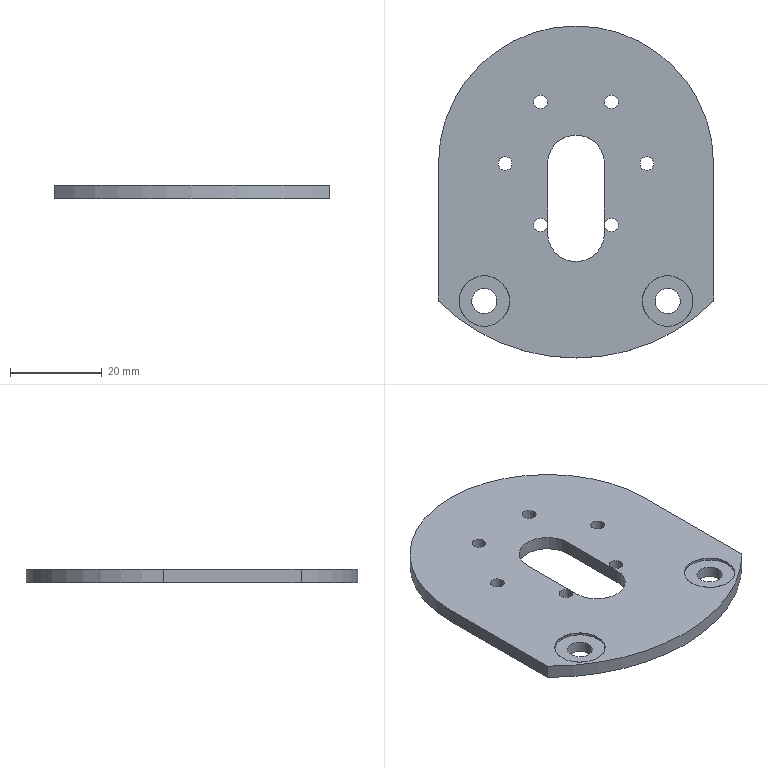Part | SolidWorks | features Extrusion 1, HoleWzd 1, ICE 1 | 1 solid | 36 faces | box 60 x 72.426 x 3 mm | volume 9913 mm3 | cylinder 24 | plane 8 | cone 4 | commonest cylinder face diameters 3 x12 5.5 x4 11 x4 12.4 x2 60 x1 84.853 x1
STEP:
#1=CARTESIAN_POINT('',(-25.5,-30.,2.975));
#2=VERTEX_POINT('',#1);
#3=CARTESIAN_POINT('',(-14.5,-30.,2.975));
#4=VERTEX_POINT('',#3);
#5=CARTESIAN_POINT('',(-20.,-30.,2.975));
#6=DIRECTION('',(0.,0.,1.));
#7=DIRECTION('',(1.,0.,0.));
#8=AXIS2_PLACEMENT_3D('',#5,#6,#7);
#9=CIRCLE('',#8,5.5);
#10=EDGE_CURVE('',#2,#4,#9,.T.);
#11=ORIENTED_EDGE('',*,*,#10,.F.);
#12=CARTESIAN_POINT('',(-25.525,-30.,3.));
#13=VERTEX_POINT('',#12);
#14=CARTESIAN_POINT('',(-25.525,-30.,3.));
#15=DIRECTION('',(-0.7071,0.,0.7071));
#16=VECTOR('',#15,1000.);
#17=LINE('',#14,#16);
#18=EDGE_CURVE('',#2,#13,#17,.T.);
#19=ORIENTED_EDGE('',*,*,#18,.T.);
#20=CARTESIAN_POINT('',(-14.475,-30.,3.));
#21=VERTEX_POINT('',#20);
#22=CARTESIAN_POINT('',(-20.,-30.,3.));
#23=DIRECTION('',(0.,0.,1.));
#24=DIRECTION('',(1.,0.,0.));
#25=AXIS2_PLACEMENT_3D('',#22,#23,#24);
#26=CIRCLE('',#25,5.525);
#27=EDGE_CURVE('',#13,#21,#26,.T.);
#28=ORIENTED_EDGE('',*,*,#27,.T.);
#29=CARTESIAN_POINT('',(-14.475,-30.,3.));
#30=DIRECTION('',(0.7071,0.,0.7071));
#31=VECTOR('',#30,1000.);
#32=LINE('',#29,#31);
#33=EDGE_CURVE('',#4,#21,#32,.T.);
#34=ORIENTED_EDGE('',*,*,#33,.F.);
#35=EDGE_LOOP('',(#11,#19,#28,#34));
#36=FACE_OUTER_BOUND('',#35,.T.);
#37=CARTESIAN_POINT('',(-20.,-30.,3.));
#38=DIRECTION('',(0.,0.,1.));
#39=DIRECTION('',(1.,0.,0.));
#40=AXIS2_PLACEMENT_3D('',#37,#38,#39);
#41=CONICAL_SURFACE('',#40,5.525,0.7854);
#42=ADVANCED_FACE('',(#36),#41,.F.);
#43=CARTESIAN_POINT('',(-25.5,-30.,2.5));
#44=VERTEX_POINT('',#43);
#45=CARTESIAN_POINT('',(-14.5,-30.,2.5));
#46=VERTEX_POINT('',#45);
#47=CARTESIAN_POINT('',(-20.,-30.,2.5));
#48=DIRECTION('',(0.,0.,1.));
#49=DIRECTION('',(1.,0.,0.));
#50=AXIS2_PLACEMENT_3D('',#47,#48,#49);
#51=CIRCLE('',#50,5.5);
#52=EDGE_CURVE('',#44,#46,#51,.T.);
#53=ORIENTED_EDGE('',*,*,#52,.F.);
#54=CARTESIAN_POINT('',(-25.5,-30.,3.));
#55=DIRECTION('',(0.,0.,1.));
#56=VECTOR('',#55,1000.);
#57=LINE('',#54,#56);
#58=EDGE_CURVE('',#44,#2,#57,.T.);
#59=ORIENTED_EDGE('',*,*,#58,.T.);
#60=ORIENTED_EDGE('',*,*,#10,.T.);
#61=CARTESIAN_POINT('',(-14.5,-30.,3.));
#62=DIRECTION('',(0.,0.,1.));
#63=VECTOR('',#62,1000.);
#64=LINE('',#61,#63);
#65=EDGE_CURVE('',#46,#4,#64,.T.);
#66=ORIENTED_EDGE('',*,*,#65,.F.);
#67=EDGE_LOOP('',(#53,#59,#60,#66));
#68=FACE_OUTER_BOUND('',#67,.T.);
#69=CARTESIAN_POINT('',(-20.,-30.,3.));
#70=DIRECTION('',(0.,0.,1.));
#71=DIRECTION('',(1.,0.,0.));
#72=AXIS2_PLACEMENT_3D('',#69,#70,#71);
#73=CYLINDRICAL_SURFACE('',#72,5.5);
#74=ADVANCED_FACE('',(#68),#73,.F.);
#75=CARTESIAN_POINT('',(-22.75,-30.,0.));
#76=VERTEX_POINT('',#75);
#77=CARTESIAN_POINT('',(-17.25,-30.,0.));
#78=VERTEX_POINT('',#77);
#79=CARTESIAN_POINT('',(-20.,-30.,0.));
#80=DIRECTION('',(0.,0.,1.));
#81=DIRECTION('',(1.,0.,0.));
#82=AXIS2_PLACEMENT_3D('',#79,#80,#81);
#83=CIRCLE('',#82,2.75);
#84=EDGE_CURVE('',#76,#78,#83,.T.);
#85=ORIENTED_EDGE('',*,*,#84,.F.);
#86=CARTESIAN_POINT('',(-22.75,-30.,2.5));
#87=VERTEX_POINT('',#86);
#88=CARTESIAN_POINT('',(-22.75,-30.,3.));
#89=DIRECTION('',(0.,0.,1.));
#90=VECTOR('',#89,1000.);
#91=LINE('',#88,#90);
#92=EDGE_CURVE('',#76,#87,#91,.T.);
#93=ORIENTED_EDGE('',*,*,#92,.T.);
#94=CARTESIAN_POINT('',(-17.25,-30.,2.5));
#95=VERTEX_POINT('',#94);
#96=CARTESIAN_POINT('',(-20.,-30.,2.5));
#97=DIRECTION('',(0.,0.,1.));
#98=DIRECTION('',(1.,0.,0.));
#99=AXIS2_PLACEMENT_3D('',#96,#97,#98);
#100=CIRCLE('',#99,2.75);
#101=EDGE_CURVE('',#87,#95,#100,.T.);
#102=ORIENTED_EDGE('',*,*,#101,.T.);
#103=CARTESIAN_POINT('',(-17.25,-30.,3.));
#104=DIRECTION('',(0.,0.,1.));
#105=VECTOR('',#104,1000.);
#106=LINE('',#103,#105);
#107=EDGE_CURVE('',#78,#95,#106,.T.);
#108=ORIENTED_EDGE('',*,*,#107,.F.);
#109=EDGE_LOOP('',(#85,#93,#102,#108));
#110=FACE_OUTER_BOUND('',#109,.T.);
#111=CARTESIAN_POINT('',(-20.,-30.,3.));
#112=DIRECTION('',(0.,0.,1.));
#113=DIRECTION('',(1.,0.,0.));
#114=AXIS2_PLACEMENT_3D('',#111,#112,#113);
#115=CYLINDRICAL_SURFACE('',#114,2.75);
#116=ADVANCED_FACE('',(#110),#115,.F.);
#117=CARTESIAN_POINT('',(14.5,-30.,2.975));
#118=VERTEX_POINT('',#117);
#119=CARTESIAN_POINT('',(25.5,-30.,2.975));
#120=VERTEX_POINT('',#119);
#121=CARTESIAN_POINT('',(20.,-30.,2.975));
#122=DIRECTION('',(0.,0.,1.));
#123=DIRECTION('',(1.,0.,0.));
#124=AXIS2_PLACEMENT_3D('',#121,#122,#123);
#125=CIRCLE('',#124,5.5);
#126=EDGE_CURVE('',#118,#120,#125,.T.);
#127=ORIENTED_EDGE('',*,*,#126,.F.);
#128=CARTESIAN_POINT('',(14.475,-30.,3.));
#129=VERTEX_POINT('',#128);
#130=CARTESIAN_POINT('',(14.475,-30.,3.));
#131=DIRECTION('',(-0.7071,0.,0.7071));
#132=VECTOR('',#131,1000.);
#133=LINE('',#130,#132);
#134=EDGE_CURVE('',#118,#129,#133,.T.);
#135=ORIENTED_EDGE('',*,*,#134,.T.);
#136=CARTESIAN_POINT('',(25.525,-30.,3.));
#137=VERTEX_POINT('',#136);
#138=CARTESIAN_POINT('',(20.,-30.,3.));
#139=DIRECTION('',(0.,0.,1.));
#140=DIRECTION('',(1.,0.,0.));
#141=AXIS2_PLACEMENT_3D('',#138,#139,#140);
#142=CIRCLE('',#141,5.525);
#143=EDGE_CURVE('',#129,#137,#142,.T.);
#144=ORIENTED_EDGE('',*,*,#143,.T.);
#145=CARTESIAN_POINT('',(25.525,-30.,3.));
#146=DIRECTION('',(0.7071,0.,0.7071));
#147=VECTOR('',#146,1000.);
#148=LINE('',#145,#147);
#149=EDGE_CURVE('',#120,#137,#148,.T.);
#150=ORIENTED_EDGE('',*,*,#149,.F.);
#151=EDGE_LOOP('',(#127,#135,#144,#150));
#152=FACE_OUTER_BOUND('',#151,.T.);
#153=CARTESIAN_POINT('',(20.,-30.,3.));
#154=DIRECTION('',(0.,0.,1.));
#155=DIRECTION('',(1.,0.,0.));
#156=AXIS2_PLACEMENT_3D('',#153,#154,#155);
#157=CONICAL_SURFACE('',#156,5.525,0.7854);
#158=ADVANCED_FACE('',(#152),#157,.F.);
#159=CARTESIAN_POINT('',(14.5,-30.,2.5));
#160=VERTEX_POINT('',#159);
#161=CARTESIAN_POINT('',(25.5,-30.,2.5));
#162=VERTEX_POINT('',#161);
#163=CARTESIAN_POINT('',(20.,-30.,2.5));
#164=DIRECTION('',(0.,0.,1.));
#165=DIRECTION('',(1.,0.,0.));
#166=AXIS2_PLACEMENT_3D('',#163,#164,#165);
#167=CIRCLE('',#166,5.5);
#168=EDGE_CURVE('',#160,#162,#167,.T.);
#169=ORIENTED_EDGE('',*,*,#168,.F.);
#170=CARTESIAN_POINT('',(14.5,-30.,3.));
#171=DIRECTION('',(0.,0.,1.));
#172=VECTOR('',#171,1000.);
#173=LINE('',#170,#172);
#174=EDGE_CURVE('',#160,#118,#173,.T.);
#175=ORIENTED_EDGE('',*,*,#174,.T.);
#176=ORIENTED_EDGE('',*,*,#126,.T.);
#177=CARTESIAN_POINT('',(25.5,-30.,3.));
#178=DIRECTION('',(0.,0.,1.));
#179=VECTOR('',#178,1000.);
#180=LINE('',#177,#179);
#181=EDGE_CURVE('',#162,#120,#180,.T.);
#182=ORIENTED_EDGE('',*,*,#181,.F.);
#183=EDGE_LOOP('',(#169,#175,#176,#182));
#184=FACE_OUTER_BOUND('',#183,.T.);
#185=CARTESIAN_POINT('',(20.,-30.,3.));
#186=DIRECTION('',(0.,0.,1.));
#187=DIRECTION('',(1.,0.,0.));
#188=AXIS2_PLACEMENT_3D('',#185,#186,#187);
#189=CYLINDRICAL_SURFACE('',#188,5.5);
#190=ADVANCED_FACE('',(#184),#189,.F.);
#191=CARTESIAN_POINT('',(17.25,-30.,0.));
#192=VERTEX_POINT('',#191);
#193=CARTESIAN_POINT('',(22.75,-30.,0.));
#194=VERTEX_POINT('',#193);
#195=CARTESIAN_POINT('',(20.,-30.,0.));
#196=DIRECTION('',(0.,0.,1.));
#197=DIRECTION('',(1.,0.,0.));
#198=AXIS2_PLACEMENT_3D('',#195,#196,#197);
#199=CIRCLE('',#198,2.75);
#200=EDGE_CURVE('',#192,#194,#199,.T.);
#201=ORIENTED_EDGE('',*,*,#200,.F.);
#202=CARTESIAN_POINT('',(17.25,-30.,2.5));
#203=VERTEX_POINT('',#202);
#204=CARTESIAN_POINT('',(17.25,-30.,3.));
#205=DIRECTION('',(0.,0.,1.));
#206=VECTOR('',#205,1000.);
#207=LINE('',#204,#206);
#208=EDGE_CURVE('',#192,#203,#207,.T.);
#209=ORIENTED_EDGE('',*,*,#208,.T.);
#210=CARTESIAN_POINT('',(22.75,-30.,2.5));
#211=VERTEX_POINT('',#210);
#212=CARTESIAN_POINT('',(20.,-30.,2.5));
#213=DIRECTION('',(0.,0.,1.));
#214=DIRECTION('',(1.,0.,0.));
#215=AXIS2_PLACEMENT_3D('',#212,#213,#214);
#216=CIRCLE('',#215,2.75);
#217=EDGE_CURVE('',#203,#211,#216,.T.);
#218=ORIENTED_EDGE('',*,*,#217,.T.);
#219=CARTESIAN_POINT('',(22.75,-30.,3.));
#220=DIRECTION('',(0.,0.,1.));
#221=VECTOR('',#220,1000.);
#222=LINE('',#219,#221);
#223=EDGE_CURVE('',#194,#211,#222,.T.);
#224=ORIENTED_EDGE('',*,*,#223,.F.);
#225=EDGE_LOOP('',(#201,#209,#218,#224));
#226=FACE_OUTER_BOUND('',#225,.T.);
#227=CARTESIAN_POINT('',(20.,-30.,3.));
#228=DIRECTION('',(0.,0.,1.));
#229=DIRECTION('',(1.,0.,0.));
#230=AXIS2_PLACEMENT_3D('',#227,#228,#229);
#231=CYLINDRICAL_SURFACE('',#230,2.75);
#232=ADVANCED_FACE('',(#226),#231,.F.);
#233=CARTESIAN_POINT('',(-16.964,0.,0.));
#234=VERTEX_POINT('',#233);
#235=CARTESIAN_POINT('',(-13.964,0.,0.));
#236=VERTEX_POINT('',#235);
#237=CARTESIAN_POINT('',(-15.464,0.,0.));
#238=DIRECTION('',(0.,0.,1.));
#239=DIRECTION('',(1.,0.,0.));
#240=AXIS2_PLACEMENT_3D('',#237,#238,#239);
#241=CIRCLE('',#240,1.5);
#242=EDGE_CURVE('',#234,#236,#241,.T.);
#243=ORIENTED_EDGE('',*,*,#242,.F.);
#244=CARTESIAN_POINT('',(-16.964,0.,3.));
#245=VERTEX_POINT('',#244);
#246=CARTESIAN_POINT('',(-16.964,0.,0.));
#247=DIRECTION('',(0.,0.,1.));
#248=VECTOR('',#247,1000.);
#249=LINE('',#246,#248);
#250=EDGE_CURVE('',#234,#245,#249,.T.);
#251=ORIENTED_EDGE('',*,*,#250,.T.);
#252=CARTESIAN_POINT('',(-13.964,0.,3.));
#253=VERTEX_POINT('',#252);
#254=CARTESIAN_POINT('',(-15.464,0.,3.));
#255=DIRECTION('',(0.,0.,1.));
#256=DIRECTION('',(1.,0.,0.));
#257=AXIS2_PLACEMENT_3D('',#254,#255,#256);
#258=CIRCLE('',#257,1.5);
#259=EDGE_CURVE('',#245,#253,#258,.T.);
#260=ORIENTED_EDGE('',*,*,#259,.T.);
#261=CARTESIAN_POINT('',(-13.964,0.,0.));
#262=DIRECTION('',(0.,0.,1.));
#263=VECTOR('',#262,1000.);
#264=LINE('',#261,#263);
#265=EDGE_CURVE('',#236,#253,#264,.T.);
#266=ORIENTED_EDGE('',*,*,#265,.F.);
#267=EDGE_LOOP('',(#243,#251,#260,#266));
#268=FACE_OUTER_BOUND('',#267,.T.);
#269=CARTESIAN_POINT('',(-15.464,0.,0.));
#270=DIRECTION('',(0.,0.,1.));
#271=DIRECTION('',(1.,0.,0.));
#272=AXIS2_PLACEMENT_3D('',#269,#270,#271);
#273=CYLINDRICAL_SURFACE('',#272,1.5);
#274=ADVANCED_FACE('',(#268),#273,.F.);
#275=CARTESIAN_POINT('',(-9.232,-13.392,0.));
#276=VERTEX_POINT('',#275);
#277=CARTESIAN_POINT('',(-6.232,-13.392,0.));
#278=VERTEX_POINT('',#277);
#279=CARTESIAN_POINT('',(-7.732,-13.392,0.));
#280=DIRECTION('',(0.,0.,1.));
#281=DIRECTION('',(1.,0.,0.));
#282=AXIS2_PLACEMENT_3D('',#279,#280,#281);
#283=CIRCLE('',#282,1.5);
#284=EDGE_CURVE('',#276,#278,#283,.T.);
#285=ORIENTED_EDGE('',*,*,#284,.F.);
#286=CARTESIAN_POINT('',(-9.232,-13.392,3.));
#287=VERTEX_POINT('',#286);
#288=CARTESIAN_POINT('',(-9.232,-13.392,0.));
#289=DIRECTION('',(0.,0.,1.));
#290=VECTOR('',#289,1000.);
#291=LINE('',#288,#290);
#292=EDGE_CURVE('',#276,#287,#291,.T.);
#293=ORIENTED_EDGE('',*,*,#292,.T.);
#294=CARTESIAN_POINT('',(-6.232,-13.392,3.));
#295=VERTEX_POINT('',#294);
#296=CARTESIAN_POINT('',(-7.732,-13.392,3.));
#297=DIRECTION('',(0.,0.,1.));
#298=DIRECTION('',(1.,0.,0.));
#299=AXIS2_PLACEMENT_3D('',#296,#297,#298);
#300=CIRCLE('',#299,1.5);
#301=EDGE_CURVE('',#287,#295,#300,.T.);
#302=ORIENTED_EDGE('',*,*,#301,.T.);
#303=CARTESIAN_POINT('',(-6.232,-13.392,0.));
#304=DIRECTION('',(0.,0.,1.));
#305=VECTOR('',#304,1000.);
#306=LINE('',#303,#305);
#307=EDGE_CURVE('',#278,#295,#306,.T.);
#308=ORIENTED_EDGE('',*,*,#307,.F.);
#309=EDGE_LOOP('',(#285,#293,#302,#308));
#310=FACE_OUTER_BOUND('',#309,.T.);
#311=CARTESIAN_POINT('',(-7.732,-13.392,0.));
#312=DIRECTION('',(0.,0.,1.));
#313=DIRECTION('',(1.,0.,0.));
#314=AXIS2_PLACEMENT_3D('',#311,#312,#313);
#315=CYLINDRICAL_SURFACE('',#314,1.5);
#316=ADVANCED_FACE('',(#310),#315,.F.);
#317=CARTESIAN_POINT('',(6.232,-13.392,0.));
#318=VERTEX_POINT('',#317);
#319=CARTESIAN_POINT('',(9.232,-13.392,0.));
#320=VERTEX_POINT('',#319);
#321=CARTESIAN_POINT('',(7.732,-13.392,0.));
#322=DIRECTION('',(0.,0.,1.));
#323=DIRECTION('',(1.,0.,0.));
#324=AXIS2_PLACEMENT_3D('',#321,#322,#323);
#325=CIRCLE('',#324,1.5);
#326=EDGE_CURVE('',#318,#320,#325,.T.);
#327=ORIENTED_EDGE('',*,*,#326,.F.);
#328=CARTESIAN_POINT('',(6.232,-13.392,3.));
#329=VERTEX_POINT('',#328);
#330=CARTESIAN_POINT('',(6.232,-13.392,0.));
#331=DIRECTION('',(0.,0.,1.));
#332=VECTOR('',#331,1000.);
#333=LINE('',#330,#332);
#334=EDGE_CURVE('',#318,#329,#333,.T.);
#335=ORIENTED_EDGE('',*,*,#334,.T.);
#336=CARTESIAN_POINT('',(9.232,-13.392,3.));
#337=VERTEX_POINT('',#336);
#338=CARTESIAN_POINT('',(7.732,-13.392,3.));
#339=DIRECTION('',(0.,0.,1.));
#340=DIRECTION('',(1.,0.,0.));
#341=AXIS2_PLACEMENT_3D('',#338,#339,#340);
#342=CIRCLE('',#341,1.5);
#343=EDGE_CURVE('',#329,#337,#342,.T.);
#344=ORIENTED_EDGE('',*,*,#343,.T.);
#345=CARTESIAN_POINT('',(9.232,-13.392,0.));
#346=DIRECTION('',(0.,0.,1.));
#347=VECTOR('',#346,1000.);
#348=LINE('',#345,#347);
#349=EDGE_CURVE('',#320,#337,#348,.T.);
#350=ORIENTED_EDGE('',*,*,#349,.F.);
#351=EDGE_LOOP('',(#327,#335,#344,#350));
#352=FACE_OUTER_BOUND('',#351,.T.);
#353=CARTESIAN_POINT('',(7.732,-13.392,0.));
#354=DIRECTION('',(0.,0.,1.));
#355=DIRECTION('',(1.,0.,0.));
#356=AXIS2_PLACEMENT_3D('',#353,#354,#355);
#357=CYLINDRICAL_SURFACE('',#356,1.5);
#358=ADVANCED_FACE('',(#352),#357,.F.);
#359=CARTESIAN_POINT('',(13.964,0.,0.));
#360=VERTEX_POINT('',#359);
#361=CARTESIAN_POINT('',(16.964,0.,0.));
#362=VERTEX_POINT('',#361);
#363=CARTESIAN_POINT('',(15.464,0.,0.));
#364=DIRECTION('',(0.,0.,1.));
#365=DIRECTION('',(1.,0.,0.));
#366=AXIS2_PLACEMENT_3D('',#363,#364,#365);
#367=CIRCLE('',#366,1.5);
#368=EDGE_CURVE('',#360,#362,#367,.T.);
#369=ORIENTED_EDGE('',*,*,#368,.F.);
#370=CARTESIAN_POINT('',(13.964,0.,3.));
#371=VERTEX_POINT('',#370);
#372=CARTESIAN_POINT('',(13.964,0.,0.));
#373=DIRECTION('',(0.,0.,1.));
#374=VECTOR('',#373,1000.);
#375=LINE('',#372,#374);
#376=EDGE_CURVE('',#360,#371,#375,.T.);
#377=ORIENTED_EDGE('',*,*,#376,.T.);
#378=CARTESIAN_POINT('',(16.964,0.,3.));
#379=VERTEX_POINT('',#378);
#380=CARTESIAN_POINT('',(15.464,0.,3.));
#381=DIRECTION('',(0.,0.,1.));
#382=DIRECTION('',(1.,0.,0.));
#383=AXIS2_PLACEMENT_3D('',#380,#381,#382);
#384=CIRCLE('',#383,1.5);
#385=EDGE_CURVE('',#371,#379,#384,.T.);
#386=ORIENTED_EDGE('',*,*,#385,.T.);
#387=CARTESIAN_POINT('',(16.964,0.,0.));
#388=DIRECTION('',(0.,0.,1.));
#389=VECTOR('',#388,1000.);
#390=LINE('',#387,#389);
#391=EDGE_CURVE('',#362,#379,#390,.T.);
#392=ORIENTED_EDGE('',*,*,#391,.F.);
#393=EDGE_LOOP('',(#369,#377,#386,#392));
#394=FACE_OUTER_BOUND('',#393,.T.);
#395=CARTESIAN_POINT('',(15.464,0.,0.));
#396=DIRECTION('',(0.,0.,1.));
#397=DIRECTION('',(1.,0.,0.));
#398=AXIS2_PLACEMENT_3D('',#395,#396,#397);
#399=CYLINDRICAL_SURFACE('',#398,1.5);
#400=ADVANCED_FACE('',(#394),#399,.F.);
#401=CARTESIAN_POINT('',(6.232,13.392,0.));
#402=VERTEX_POINT('',#401);
#403=CARTESIAN_POINT('',(9.232,13.392,0.));
#404=VERTEX_POINT('',#403);
#405=CARTESIAN_POINT('',(7.732,13.392,0.));
#406=DIRECTION('',(0.,0.,1.));
#407=DIRECTION('',(1.,0.,0.));
#408=AXIS2_PLACEMENT_3D('',#405,#406,#407);
#409=CIRCLE('',#408,1.5);
#410=EDGE_CURVE('',#402,#404,#409,.T.);
#411=ORIENTED_EDGE('',*,*,#410,.F.);
#412=CARTESIAN_POINT('',(6.232,13.392,3.));
#413=VERTEX_POINT('',#412);
#414=CARTESIAN_POINT('',(6.232,13.392,0.));
#415=DIRECTION('',(0.,0.,1.));
#416=VECTOR('',#415,1000.);
#417=LINE('',#414,#416);
#418=EDGE_CURVE('',#402,#413,#417,.T.);
#419=ORIENTED_EDGE('',*,*,#418,.T.);
#420=CARTESIAN_POINT('',(9.232,13.392,3.));
#421=VERTEX_POINT('',#420);
#422=CARTESIAN_POINT('',(7.732,13.392,3.));
#423=DIRECTION('',(0.,0.,1.));
#424=DIRECTION('',(1.,0.,0.));
#425=AXIS2_PLACEMENT_3D('',#422,#423,#424);
#426=CIRCLE('',#425,1.5);
#427=EDGE_CURVE('',#413,#421,#426,.T.);
#428=ORIENTED_EDGE('',*,*,#427,.T.);
#429=CARTESIAN_POINT('',(9.232,13.392,0.));
#430=DIRECTION('',(0.,0.,1.));
#431=VECTOR('',#430,1000.);
#432=LINE('',#429,#431);
#433=EDGE_CURVE('',#404,#421,#432,.T.);
#434=ORIENTED_EDGE('',*,*,#433,.F.);
#435=EDGE_LOOP('',(#411,#419,#428,#434));
#436=FACE_OUTER_BOUND('',#435,.T.);
#437=CARTESIAN_POINT('',(7.732,13.392,0.));
#438=DIRECTION('',(0.,0.,1.));
#439=DIRECTION('',(1.,0.,0.));
#440=AXIS2_PLACEMENT_3D('',#437,#438,#439);
#441=CYLINDRICAL_SURFACE('',#440,1.5);
#442=ADVANCED_FACE('',(#436),#441,.F.);
#443=CARTESIAN_POINT('',(-9.232,13.392,0.));
#444=VERTEX_POINT('',#443);
#445=CARTESIAN_POINT('',(-6.232,13.392,0.));
#446=VERTEX_POINT('',#445);
#447=CARTESIAN_POINT('',(-7.732,13.392,0.));
#448=DIRECTION('',(0.,0.,1.));
#449=DIRECTION('',(1.,0.,0.));
#450=AXIS2_PLACEMENT_3D('',#447,#448,#449);
#451=CIRCLE('',#450,1.5);
#452=EDGE_CURVE('',#444,#446,#451,.T.);
#453=ORIENTED_EDGE('',*,*,#452,.F.);
#454=CARTESIAN_POINT('',(-9.232,13.392,3.));
#455=VERTEX_POINT('',#454);
#456=CARTESIAN_POINT('',(-9.232,13.392,0.));
#457=DIRECTION('',(0.,0.,1.));
#458=VECTOR('',#457,1000.);
#459=LINE('',#456,#458);
#460=EDGE_CURVE('',#444,#455,#459,.T.);
#461=ORIENTED_EDGE('',*,*,#460,.T.);
#462=CARTESIAN_POINT('',(-6.232,13.392,3.));
#463=VERTEX_POINT('',#462);
#464=CARTESIAN_POINT('',(-7.732,13.392,3.));
#465=DIRECTION('',(0.,0.,1.));
#466=DIRECTION('',(1.,0.,0.));
#467=AXIS2_PLACEMENT_3D('',#464,#465,#466);
#468=CIRCLE('',#467,1.5);
#469=EDGE_CURVE('',#455,#463,#468,.T.);
#470=ORIENTED_EDGE('',*,*,#469,.T.);
#471=CARTESIAN_POINT('',(-6.232,13.392,0.));
#472=DIRECTION('',(0.,0.,1.));
#473=VECTOR('',#472,1000.);
#474=LINE('',#471,#473);
#475=EDGE_CURVE('',#446,#463,#474,.T.);
#476=ORIENTED_EDGE('',*,*,#475,.F.);
#477=EDGE_LOOP('',(#453,#461,#470,#476));
#478=FACE_OUTER_BOUND('',#477,.T.);
#479=CARTESIAN_POINT('',(-7.732,13.392,0.));
#480=DIRECTION('',(0.,0.,1.));
#481=DIRECTION('',(1.,0.,0.));
#482=AXIS2_PLACEMENT_3D('',#479,#480,#481);
#483=CYLINDRICAL_SURFACE('',#482,1.5);
#484=ADVANCED_FACE('',(#478),#483,.F.);
#485=CARTESIAN_POINT('',(-20.,-30.,3.));
#486=DIRECTION('',(0.,0.,1.));
#487=DIRECTION('',(1.,0.,0.));
#488=AXIS2_PLACEMENT_3D('',#485,#486,#487);
#489=CIRCLE('',#488,5.525);
#490=EDGE_CURVE('',#21,#13,#489,.T.);
#491=ORIENTED_EDGE('',*,*,#490,.F.);
#492=ORIENTED_EDGE('',*,*,#27,.F.);
#493=EDGE_LOOP('',(#491,#492));
#494=FACE_BOUND('',#493,.T.);
#495=CARTESIAN_POINT('',(20.,-30.,3.));
#496=DIRECTION('',(0.,0.,1.));
#497=DIRECTION('',(1.,0.,0.));
#498=AXIS2_PLACEMENT_3D('',#495,#496,#497);
#499=CIRCLE('',#498,5.525);
#500=EDGE_CURVE('',#137,#129,#499,.T.);
#501=ORIENTED_EDGE('',*,*,#500,.F.);
#502=ORIENTED_EDGE('',*,*,#143,.F.);
#503=EDGE_LOOP('',(#501,#502));
#504=FACE_BOUND('',#503,.T.);
#505=CARTESIAN_POINT('',(-15.464,0.,3.));
#506=DIRECTION('',(0.,0.,1.));
#507=DIRECTION('',(1.,0.,0.));
#508=AXIS2_PLACEMENT_3D('',#505,#506,#507);
#509=CIRCLE('',#508,1.5);
#510=EDGE_CURVE('',#253,#245,#509,.T.);
#511=ORIENTED_EDGE('',*,*,#510,.F.);
#512=ORIENTED_EDGE('',*,*,#259,.F.);
#513=EDGE_LOOP('',(#511,#512));
#514=FACE_BOUND('',#513,.T.);
#515=CARTESIAN_POINT('',(-7.732,-13.392,3.));
#516=DIRECTION('',(0.,0.,1.));
#517=DIRECTION('',(1.,0.,0.));
#518=AXIS2_PLACEMENT_3D('',#515,#516,#517);
#519=CIRCLE('',#518,1.5);
#520=EDGE_CURVE('',#295,#287,#519,.T.);
#521=ORIENTED_EDGE('',*,*,#520,.F.);
#522=ORIENTED_EDGE('',*,*,#301,.F.);
#523=EDGE_LOOP('',(#521,#522));
#524=FACE_BOUND('',#523,.T.);
#525=CARTESIAN_POINT('',(7.732,-13.392,3.));
#526=DIRECTION('',(0.,0.,1.));
#527=DIRECTION('',(1.,0.,0.));
#528=AXIS2_PLACEMENT_3D('',#525,#526,#527);
#529=CIRCLE('',#528,1.5);
#530=EDGE_CURVE('',#337,#329,#529,.T.);
#531=ORIENTED_EDGE('',*,*,#530,.F.);
#532=ORIENTED_EDGE('',*,*,#343,.F.);
#533=EDGE_LOOP('',(#531,#532));
#534=FACE_BOUND('',#533,.T.);
#535=CARTESIAN_POINT('',(15.464,0.,3.));
#536=DIRECTION('',(0.,0.,1.));
#537=DIRECTION('',(1.,0.,0.));
#538=AXIS2_PLACEMENT_3D('',#535,#536,#537);
#539=CIRCLE('',#538,1.5);
#540=EDGE_CURVE('',#379,#371,#539,.T.);
#541=ORIENTED_EDGE('',*,*,#540,.F.);
#542=ORIENTED_EDGE('',*,*,#385,.F.);
#543=EDGE_LOOP('',(#541,#542));
#544=FACE_BOUND('',#543,.T.);
#545=CARTESIAN_POINT('',(7.732,13.392,3.));
#546=DIRECTION('',(0.,0.,1.));
#547=DIRECTION('',(1.,0.,0.));
#548=AXIS2_PLACEMENT_3D('',#545,#546,#547);
#549=CIRCLE('',#548,1.5);
#550=EDGE_CURVE('',#421,#413,#549,.T.);
#551=ORIENTED_EDGE('',*,*,#550,.F.);
#552=ORIENTED_EDGE('',*,*,#427,.F.);
#553=EDGE_LOOP('',(#551,#552));
#554=FACE_BOUND('',#553,.T.);
#555=CARTESIAN_POINT('',(-7.732,13.392,3.));
#556=DIRECTION('',(0.,0.,1.));
#557=DIRECTION('',(1.,0.,0.));
#558=AXIS2_PLACEMENT_3D('',#555,#556,#557);
#559=CIRCLE('',#558,1.5);
#560=EDGE_CURVE('',#463,#455,#559,.T.);
#561=ORIENTED_EDGE('',*,*,#560,.F.);
#562=ORIENTED_EDGE('',*,*,#469,.F.);
#563=EDGE_LOOP('',(#561,#562));
#564=FACE_BOUND('',#563,.T.);
#565=CARTESIAN_POINT('',(30.,0.,3.));
#566=VERTEX_POINT('',#565);
#567=CARTESIAN_POINT('',(-30.,0.,3.));
#568=VERTEX_POINT('',#567);
#569=CARTESIAN_POINT('',(0.,0.,3.));
#570=DIRECTION('',(0.,0.,1.));
#571=DIRECTION('',(1.,0.,0.));
#572=AXIS2_PLACEMENT_3D('',#569,#570,#571);
#573=CIRCLE('',#572,30.);
#574=EDGE_CURVE('',#566,#568,#573,.T.);
#575=ORIENTED_EDGE('',*,*,#574,.T.);
#576=CARTESIAN_POINT('',(-30.,-30.,3.));
#577=VERTEX_POINT('',#576);
#578=CARTESIAN_POINT('',(-30.,0.,3.));
#579=DIRECTION('',(0.,-1.,0.));
#580=VECTOR('',#579,1000.);
#581=LINE('',#578,#580);
#582=EDGE_CURVE('',#568,#577,#581,.T.);
#583=ORIENTED_EDGE('',*,*,#582,.T.);
#584=CARTESIAN_POINT('',(30.,-30.,3.));
#585=VERTEX_POINT('',#584);
#586=CARTESIAN_POINT('',(0.,0.,3.));
#587=DIRECTION('',(0.,0.,1.));
#588=DIRECTION('',(1.,0.,0.));
#589=AXIS2_PLACEMENT_3D('',#586,#587,#588);
#590=CIRCLE('',#589,42.426);
#591=EDGE_CURVE('',#577,#585,#590,.T.);
#592=ORIENTED_EDGE('',*,*,#591,.T.);
#593=CARTESIAN_POINT('',(30.,0.,3.));
#594=DIRECTION('',(0.,1.,0.));
#595=VECTOR('',#594,1000.);
#596=LINE('',#593,#595);
#597=EDGE_CURVE('',#585,#566,#596,.T.);
#598=ORIENTED_EDGE('',*,*,#597,.T.);
#599=EDGE_LOOP('',(#575,#583,#592,#598));
#600=FACE_OUTER_BOUND('',#599,.T.);
#601=CARTESIAN_POINT('',(-6.2,0.,3.));
#602=VERTEX_POINT('',#601);
#603=CARTESIAN_POINT('',(-6.2,-15.219,3.));
#604=VERTEX_POINT('',#603);
#605=CARTESIAN_POINT('',(-6.2,0.,3.));
#606=DIRECTION('',(0.,-1.,0.));
#607=VECTOR('',#606,1000.);
#608=LINE('',#605,#607);
#609=EDGE_CURVE('',#602,#604,#608,.T.);
#610=ORIENTED_EDGE('',*,*,#609,.F.);
#611=CARTESIAN_POINT('',(6.2,0.,3.));
#612=VERTEX_POINT('',#611);
#613=CARTESIAN_POINT('',(0.,0.,3.));
#614=DIRECTION('',(0.,0.,1.));
#615=DIRECTION('',(1.,0.,0.));
#616=AXIS2_PLACEMENT_3D('',#613,#614,#615);
#617=CIRCLE('',#616,6.2);
#618=EDGE_CURVE('',#612,#602,#617,.T.);
#619=ORIENTED_EDGE('',*,*,#618,.F.);
#620=CARTESIAN_POINT('',(6.2,-15.219,3.));
#621=VERTEX_POINT('',#620);
#622=CARTESIAN_POINT('',(6.2,0.,3.));
#623=DIRECTION('',(0.,1.,0.));
#624=VECTOR('',#623,1000.);
#625=LINE('',#622,#624);
#626=EDGE_CURVE('',#621,#612,#625,.T.);
#627=ORIENTED_EDGE('',*,*,#626,.F.);
#628=CARTESIAN_POINT('',(0.,-15.219,3.));
#629=DIRECTION('',(0.,0.,1.));
#630=DIRECTION('',(1.,0.,0.));
#631=AXIS2_PLACEMENT_3D('',#628,#629,#630);
#632=CIRCLE('',#631,6.2);
#633=EDGE_CURVE('',#604,#621,#632,.T.);
#634=ORIENTED_EDGE('',*,*,#633,.F.);
#635=EDGE_LOOP('',(#610,#619,#627,#634));
#636=FACE_BOUND('',#635,.T.);
#637=CARTESIAN_POINT('',(0.,0.,3.));
#638=DIRECTION('',(0.,0.,1.));
#639=DIRECTION('',(1.,0.,0.));
#640=AXIS2_PLACEMENT_3D('',#637,#638,#639);
#641=PLANE('',#640);
#642=ADVANCED_FACE('',(#494,#504,#514,#524,#534,#544,#554,#564,#600,#636),#641,.T.);
#643=CARTESIAN_POINT('',(-20.,-30.,0.));
#644=DIRECTION('',(0.,0.,1.));
#645=DIRECTION('',(1.,0.,0.));
#646=AXIS2_PLACEMENT_3D('',#643,#644,#645);
#647=CIRCLE('',#646,2.75);
#648=EDGE_CURVE('',#78,#76,#647,.T.);
#649=ORIENTED_EDGE('',*,*,#648,.T.);
#650=ORIENTED_EDGE('',*,*,#84,.T.);
#651=EDGE_LOOP('',(#649,#650));
#652=FACE_BOUND('',#651,.T.);
#653=CARTESIAN_POINT('',(20.,-30.,0.));
#654=DIRECTION('',(0.,0.,1.));
#655=DIRECTION('',(1.,0.,0.));
#656=AXIS2_PLACEMENT_3D('',#653,#654,#655);
#657=CIRCLE('',#656,2.75);
#658=EDGE_CURVE('',#194,#192,#657,.T.);
#659=ORIENTED_EDGE('',*,*,#658,.T.);
#660=ORIENTED_EDGE('',*,*,#200,.T.);
#661=EDGE_LOOP('',(#659,#660));
#662=FACE_BOUND('',#661,.T.);
#663=CARTESIAN_POINT('',(-15.464,0.,0.));
#664=DIRECTION('',(0.,0.,1.));
#665=DIRECTION('',(1.,0.,0.));
#666=AXIS2_PLACEMENT_3D('',#663,#664,#665);
#667=CIRCLE('',#666,1.5);
#668=EDGE_CURVE('',#236,#234,#667,.T.);
#669=ORIENTED_EDGE('',*,*,#668,.T.);
#670=ORIENTED_EDGE('',*,*,#242,.T.);
#671=EDGE_LOOP('',(#669,#670));
#672=FACE_BOUND('',#671,.T.);
#673=CARTESIAN_POINT('',(-7.732,-13.392,0.));
#674=DIRECTION('',(0.,0.,1.));
#675=DIRECTION('',(1.,0.,0.));
#676=AXIS2_PLACEMENT_3D('',#673,#674,#675);
#677=CIRCLE('',#676,1.5);
#678=EDGE_CURVE('',#278,#276,#677,.T.);
#679=ORIENTED_EDGE('',*,*,#678,.T.);
#680=ORIENTED_EDGE('',*,*,#284,.T.);
#681=EDGE_LOOP('',(#679,#680));
#682=FACE_BOUND('',#681,.T.);
#683=CARTESIAN_POINT('',(7.732,-13.392,0.));
#684=DIRECTION('',(0.,0.,1.));
#685=DIRECTION('',(1.,0.,0.));
#686=AXIS2_PLACEMENT_3D('',#683,#684,#685);
#687=CIRCLE('',#686,1.5);
#688=EDGE_CURVE('',#320,#318,#687,.T.);
#689=ORIENTED_EDGE('',*,*,#688,.T.);
#690=ORIENTED_EDGE('',*,*,#326,.T.);
#691=EDGE_LOOP('',(#689,#690));
#692=FACE_BOUND('',#691,.T.);
#693=CARTESIAN_POINT('',(15.464,0.,0.));
#694=DIRECTION('',(0.,0.,1.));
#695=DIRECTION('',(1.,0.,0.));
#696=AXIS2_PLACEMENT_3D('',#693,#694,#695);
#697=CIRCLE('',#696,1.5);
#698=EDGE_CURVE('',#362,#360,#697,.T.);
#699=ORIENTED_EDGE('',*,*,#698,.T.);
#700=ORIENTED_EDGE('',*,*,#368,.T.);
#701=EDGE_LOOP('',(#699,#700));
#702=FACE_BOUND('',#701,.T.);
#703=CARTESIAN_POINT('',(7.732,13.392,0.));
#704=DIRECTION('',(0.,0.,1.));
#705=DIRECTION('',(1.,0.,0.));
#706=AXIS2_PLACEMENT_3D('',#703,#704,#705);
#707=CIRCLE('',#706,1.5);
#708=EDGE_CURVE('',#404,#402,#707,.T.);
#709=ORIENTED_EDGE('',*,*,#708,.T.);
#710=ORIENTED_EDGE('',*,*,#410,.T.);
#711=EDGE_LOOP('',(#709,#710));
#712=FACE_BOUND('',#711,.T.);
#713=CARTESIAN_POINT('',(-7.732,13.392,0.));
#714=DIRECTION('',(0.,0.,1.));
#715=DIRECTION('',(1.,0.,0.));
#716=AXIS2_PLACEMENT_3D('',#713,#714,#715);
#717=CIRCLE('',#716,1.5);
#718=EDGE_CURVE('',#446,#444,#717,.T.);
#719=ORIENTED_EDGE('',*,*,#718,.T.);
#720=ORIENTED_EDGE('',*,*,#452,.T.);
#721=EDGE_LOOP('',(#719,#720));
#722=FACE_BOUND('',#721,.T.);
#723=CARTESIAN_POINT('',(30.,0.,0.));
#724=VERTEX_POINT('',#723);
#725=CARTESIAN_POINT('',(-30.,0.,0.));
#726=VERTEX_POINT('',#725);
#727=CARTESIAN_POINT('',(0.,0.,0.));
#728=DIRECTION('',(0.,0.,1.));
#729=DIRECTION('',(1.,0.,0.));
#730=AXIS2_PLACEMENT_3D('',#727,#728,#729);
#731=CIRCLE('',#730,30.);
#732=EDGE_CURVE('',#724,#726,#731,.T.);
#733=ORIENTED_EDGE('',*,*,#732,.F.);
#734=CARTESIAN_POINT('',(30.,-30.,0.));
#735=VERTEX_POINT('',#734);
#736=CARTESIAN_POINT('',(30.,0.,0.));
#737=DIRECTION('',(0.,1.,0.));
#738=VECTOR('',#737,1000.);
#739=LINE('',#736,#738);
#740=EDGE_CURVE('',#735,#724,#739,.T.);
#741=ORIENTED_EDGE('',*,*,#740,.F.);
#742=CARTESIAN_POINT('',(-30.,-30.,0.));
#743=VERTEX_POINT('',#742);
#744=CARTESIAN_POINT('',(0.,0.,0.));
#745=DIRECTION('',(0.,0.,1.));
#746=DIRECTION('',(1.,0.,0.));
#747=AXIS2_PLACEMENT_3D('',#744,#745,#746);
#748=CIRCLE('',#747,42.426);
#749=EDGE_CURVE('',#743,#735,#748,.T.);
#750=ORIENTED_EDGE('',*,*,#749,.F.);
#751=CARTESIAN_POINT('',(-30.,0.,0.));
#752=DIRECTION('',(0.,-1.,0.));
#753=VECTOR('',#752,1000.);
#754=LINE('',#751,#753);
#755=EDGE_CURVE('',#726,#743,#754,.T.);
#756=ORIENTED_EDGE('',*,*,#755,.F.);
#757=EDGE_LOOP('',(#733,#741,#750,#756));
#758=FACE_OUTER_BOUND('',#757,.T.);
#759=CARTESIAN_POINT('',(6.2,0.,0.));
#760=VERTEX_POINT('',#759);
#761=CARTESIAN_POINT('',(-6.2,0.,0.));
#762=VERTEX_POINT('',#761);
#763=CARTESIAN_POINT('',(0.,0.,0.));
#764=DIRECTION('',(0.,0.,1.));
#765=DIRECTION('',(1.,0.,0.));
#766=AXIS2_PLACEMENT_3D('',#763,#764,#765);
#767=CIRCLE('',#766,6.2);
#768=EDGE_CURVE('',#760,#762,#767,.T.);
#769=ORIENTED_EDGE('',*,*,#768,.T.);
#770=CARTESIAN_POINT('',(-6.2,-15.219,0.));
#771=VERTEX_POINT('',#770);
#772=CARTESIAN_POINT('',(-6.2,0.,0.));
#773=DIRECTION('',(0.,-1.,0.));
#774=VECTOR('',#773,1000.);
#775=LINE('',#772,#774);
#776=EDGE_CURVE('',#762,#771,#775,.T.);
#777=ORIENTED_EDGE('',*,*,#776,.T.);
#778=CARTESIAN_POINT('',(6.2,-15.219,0.));
#779=VERTEX_POINT('',#778);
#780=CARTESIAN_POINT('',(0.,-15.219,0.));
#781=DIRECTION('',(0.,0.,1.));
#782=DIRECTION('',(1.,0.,0.));
#783=AXIS2_PLACEMENT_3D('',#780,#781,#782);
#784=CIRCLE('',#783,6.2);
#785=EDGE_CURVE('',#771,#779,#784,.T.);
#786=ORIENTED_EDGE('',*,*,#785,.T.);
#787=CARTESIAN_POINT('',(6.2,0.,0.));
#788=DIRECTION('',(0.,1.,0.));
#789=VECTOR('',#788,1000.);
#790=LINE('',#787,#789);
#791=EDGE_CURVE('',#779,#760,#790,.T.);
#792=ORIENTED_EDGE('',*,*,#791,.T.);
#793=EDGE_LOOP('',(#769,#777,#786,#792));
#794=FACE_BOUND('',#793,.T.);
#795=CARTESIAN_POINT('',(0.,0.,0.));
#796=DIRECTION('',(0.,0.,1.));
#797=DIRECTION('',(1.,0.,0.));
#798=AXIS2_PLACEMENT_3D('',#795,#796,#797);
#799=PLANE('',#798);
#800=ADVANCED_FACE('',(#652,#662,#672,#682,#692,#702,#712,#722,#758,#794),#799,.F.);
#801=ORIENTED_EDGE('',*,*,#732,.T.);
#802=CARTESIAN_POINT('',(-30.,0.,3.));
#803=DIRECTION('',(0.,0.,-1.));
#804=VECTOR('',#803,1000.);
#805=LINE('',#802,#804);
#806=EDGE_CURVE('',#568,#726,#805,.T.);
#807=ORIENTED_EDGE('',*,*,#806,.F.);
#808=ORIENTED_EDGE('',*,*,#574,.F.);
#809=CARTESIAN_POINT('',(30.,0.,3.));
#810=DIRECTION('',(0.,0.,-1.));
#811=VECTOR('',#810,1000.);
#812=LINE('',#809,#811);
#813=EDGE_CURVE('',#566,#724,#812,.T.);
#814=ORIENTED_EDGE('',*,*,#813,.T.);
#815=EDGE_LOOP('',(#801,#807,#808,#814));
#816=FACE_OUTER_BOUND('',#815,.T.);
#817=CARTESIAN_POINT('',(0.,0.,3.));
#818=DIRECTION('',(0.,0.,-1.));
#819=DIRECTION('',(-1.,0.,0.));
#820=AXIS2_PLACEMENT_3D('',#817,#818,#819);
#821=CYLINDRICAL_SURFACE('',#820,30.);
#822=ADVANCED_FACE('',(#816),#821,.T.);
#823=ORIENTED_EDGE('',*,*,#755,.T.);
#824=CARTESIAN_POINT('',(-30.,-30.,3.));
#825=DIRECTION('',(0.,0.,-1.));
#826=VECTOR('',#825,1000.);
#827=LINE('',#824,#826);
#828=EDGE_CURVE('',#577,#743,#827,.T.);
#829=ORIENTED_EDGE('',*,*,#828,.F.);
#830=ORIENTED_EDGE('',*,*,#582,.F.);
#831=ORIENTED_EDGE('',*,*,#806,.T.);
#832=EDGE_LOOP('',(#823,#829,#830,#831));
#833=FACE_OUTER_BOUND('',#832,.T.);
#834=CARTESIAN_POINT('',(-30.,0.,3.));
#835=DIRECTION('',(1.,0.,0.));
#836=DIRECTION('',(0.,0.,-1.));
#837=AXIS2_PLACEMENT_3D('',#834,#835,#836);
#838=PLANE('',#837);
#839=ADVANCED_FACE('',(#833),#838,.F.);
#840=ORIENTED_EDGE('',*,*,#749,.T.);
#841=CARTESIAN_POINT('',(30.,-30.,3.));
#842=DIRECTION('',(0.,0.,-1.));
#843=VECTOR('',#842,1000.);
#844=LINE('',#841,#843);
#845=EDGE_CURVE('',#585,#735,#844,.T.);
#846=ORIENTED_EDGE('',*,*,#845,.F.);
#847=ORIENTED_EDGE('',*,*,#591,.F.);
#848=ORIENTED_EDGE('',*,*,#828,.T.);
#849=EDGE_LOOP('',(#840,#846,#847,#848));
#850=FACE_OUTER_BOUND('',#849,.T.);
#851=CARTESIAN_POINT('',(0.,0.,3.));
#852=DIRECTION('',(0.,0.,-1.));
#853=DIRECTION('',(-1.,0.,0.));
#854=AXIS2_PLACEMENT_3D('',#851,#852,#853);
#855=CYLINDRICAL_SURFACE('',#854,42.426);
#856=ADVANCED_FACE('',(#850),#855,.T.);
#857=ORIENTED_EDGE('',*,*,#740,.T.);
#858=ORIENTED_EDGE('',*,*,#813,.F.);
#859=ORIENTED_EDGE('',*,*,#597,.F.);
#860=ORIENTED_EDGE('',*,*,#845,.T.);
#861=EDGE_LOOP('',(#857,#858,#859,#860));
#862=FACE_OUTER_BOUND('',#861,.T.);
#863=CARTESIAN_POINT('',(30.,0.,3.));
#864=DIRECTION('',(-1.,0.,0.));
#865=DIRECTION('',(0.,-1.,0.));
#866=AXIS2_PLACEMENT_3D('',#863,#864,#865);
#867=PLANE('',#866);
#868=ADVANCED_FACE('',(#862),#867,.F.);
#869=ORIENTED_EDGE('',*,*,#768,.F.);
#870=CARTESIAN_POINT('',(6.2,0.,3.));
#871=DIRECTION('',(0.,0.,-1.));
#872=VECTOR('',#871,1000.);
#873=LINE('',#870,#872);
#874=EDGE_CURVE('',#612,#760,#873,.T.);
#875=ORIENTED_EDGE('',*,*,#874,.F.);
#876=ORIENTED_EDGE('',*,*,#618,.T.);
#877=CARTESIAN_POINT('',(-6.2,0.,3.));
#878=DIRECTION('',(0.,0.,-1.));
#879=VECTOR('',#878,1000.);
#880=LINE('',#877,#879);
#881=EDGE_CURVE('',#602,#762,#880,.T.);
#882=ORIENTED_EDGE('',*,*,#881,.T.);
#883=EDGE_LOOP('',(#869,#875,#876,#882));
#884=FACE_OUTER_BOUND('',#883,.T.);
#885=CARTESIAN_POINT('',(0.,0.,3.));
#886=DIRECTION('',(0.,0.,-1.));
#887=DIRECTION('',(-1.,0.,0.));
#888=AXIS2_PLACEMENT_3D('',#885,#886,#887);
#889=CYLINDRICAL_SURFACE('',#888,6.2);
#890=ADVANCED_FACE('',(#884),#889,.F.);
#891=ORIENTED_EDGE('',*,*,#776,.F.);
#892=ORIENTED_EDGE('',*,*,#881,.F.);
#893=ORIENTED_EDGE('',*,*,#609,.T.);
#894=CARTESIAN_POINT('',(-6.2,-15.219,3.));
#895=DIRECTION('',(0.,0.,-1.));
#896=VECTOR('',#895,1000.);
#897=LINE('',#894,#896);
#898=EDGE_CURVE('',#604,#771,#897,.T.);
#899=ORIENTED_EDGE('',*,*,#898,.T.);
#900=EDGE_LOOP('',(#891,#892,#893,#899));
#901=FACE_OUTER_BOUND('',#900,.T.);
#902=CARTESIAN_POINT('',(-6.2,0.,3.));
#903=DIRECTION('',(1.,0.,0.));
#904=DIRECTION('',(0.,1.,0.));
#905=AXIS2_PLACEMENT_3D('',#902,#903,#904);
#906=PLANE('',#905);
#907=ADVANCED_FACE('',(#901),#906,.T.);
#908=ORIENTED_EDGE('',*,*,#785,.F.);
#909=ORIENTED_EDGE('',*,*,#898,.F.);
#910=ORIENTED_EDGE('',*,*,#633,.T.);
#911=CARTESIAN_POINT('',(6.2,-15.219,3.));
#912=DIRECTION('',(0.,0.,-1.));
#913=VECTOR('',#912,1000.);
#914=LINE('',#911,#913);
#915=EDGE_CURVE('',#621,#779,#914,.T.);
#916=ORIENTED_EDGE('',*,*,#915,.T.);
#917=EDGE_LOOP('',(#908,#909,#910,#916));
#918=FACE_OUTER_BOUND('',#917,.T.);
#919=CARTESIAN_POINT('',(0.,-15.219,3.));
#920=DIRECTION('',(0.,0.,-1.));
#921=DIRECTION('',(-1.,0.,0.));
#922=AXIS2_PLACEMENT_3D('',#919,#920,#921);
#923=CYLINDRICAL_SURFACE('',#922,6.2);
#924=ADVANCED_FACE('',(#918),#923,.F.);
#925=ORIENTED_EDGE('',*,*,#791,.F.);
#926=ORIENTED_EDGE('',*,*,#915,.F.);
#927=ORIENTED_EDGE('',*,*,#626,.T.);
#928=ORIENTED_EDGE('',*,*,#874,.T.);
#929=EDGE_LOOP('',(#925,#926,#927,#928));
#930=FACE_OUTER_BOUND('',#929,.T.);
#931=CARTESIAN_POINT('',(6.2,0.,3.));
#932=DIRECTION('',(-1.,0.,0.));
#933=DIRECTION('',(0.,-1.,0.));
#934=AXIS2_PLACEMENT_3D('',#931,#932,#933);
#935=PLANE('',#934);
#936=ADVANCED_FACE('',(#930),#935,.T.);
#937=ORIENTED_EDGE('',*,*,#460,.F.);
#938=ORIENTED_EDGE('',*,*,#718,.F.);
#939=ORIENTED_EDGE('',*,*,#475,.T.);
#940=ORIENTED_EDGE('',*,*,#560,.T.);
#941=EDGE_LOOP('',(#937,#938,#939,#940));
#942=FACE_OUTER_BOUND('',#941,.T.);
#943=CARTESIAN_POINT('',(-7.732,13.392,0.));
#944=DIRECTION('',(0.,0.,1.));
#945=DIRECTION('',(1.,0.,0.));
#946=AXIS2_PLACEMENT_3D('',#943,#944,#945);
#947=CYLINDRICAL_SURFACE('',#946,1.5);
#948=ADVANCED_FACE('',(#942),#947,.F.);
#949=ORIENTED_EDGE('',*,*,#418,.F.);
#950=ORIENTED_EDGE('',*,*,#708,.F.);
#951=ORIENTED_EDGE('',*,*,#433,.T.);
#952=ORIENTED_EDGE('',*,*,#550,.T.);
#953=EDGE_LOOP('',(#949,#950,#951,#952));
#954=FACE_OUTER_BOUND('',#953,.T.);
#955=CARTESIAN_POINT('',(7.732,13.392,0.));
#956=DIRECTION('',(0.,0.,1.));
#957=DIRECTION('',(1.,0.,0.));
#958=AXIS2_PLACEMENT_3D('',#955,#956,#957);
#959=CYLINDRICAL_SURFACE('',#958,1.5);
#960=ADVANCED_FACE('',(#954),#959,.F.);
#961=ORIENTED_EDGE('',*,*,#376,.F.);
#962=ORIENTED_EDGE('',*,*,#698,.F.);
#963=ORIENTED_EDGE('',*,*,#391,.T.);
#964=ORIENTED_EDGE('',*,*,#540,.T.);
#965=EDGE_LOOP('',(#961,#962,#963,#964));
#966=FACE_OUTER_BOUND('',#965,.T.);
#967=CARTESIAN_POINT('',(15.464,0.,0.));
#968=DIRECTION('',(0.,0.,1.));
#969=DIRECTION('',(1.,0.,0.));
#970=AXIS2_PLACEMENT_3D('',#967,#968,#969);
#971=CYLINDRICAL_SURFACE('',#970,1.5);
#972=ADVANCED_FACE('',(#966),#971,.F.);
#973=ORIENTED_EDGE('',*,*,#334,.F.);
#974=ORIENTED_EDGE('',*,*,#688,.F.);
#975=ORIENTED_EDGE('',*,*,#349,.T.);
#976=ORIENTED_EDGE('',*,*,#530,.T.);
#977=EDGE_LOOP('',(#973,#974,#975,#976));
#978=FACE_OUTER_BOUND('',#977,.T.);
#979=CARTESIAN_POINT('',(7.732,-13.392,0.));
#980=DIRECTION('',(0.,0.,1.));
#981=DIRECTION('',(1.,0.,0.));
#982=AXIS2_PLACEMENT_3D('',#979,#980,#981);
#983=CYLINDRICAL_SURFACE('',#982,1.5);
#984=ADVANCED_FACE('',(#978),#983,.F.);
#985=ORIENTED_EDGE('',*,*,#292,.F.);
#986=ORIENTED_EDGE('',*,*,#678,.F.);
#987=ORIENTED_EDGE('',*,*,#307,.T.);
#988=ORIENTED_EDGE('',*,*,#520,.T.);
#989=EDGE_LOOP('',(#985,#986,#987,#988));
#990=FACE_OUTER_BOUND('',#989,.T.);
#991=CARTESIAN_POINT('',(-7.732,-13.392,0.));
#992=DIRECTION('',(0.,0.,1.));
#993=DIRECTION('',(1.,0.,0.));
#994=AXIS2_PLACEMENT_3D('',#991,#992,#993);
#995=CYLINDRICAL_SURFACE('',#994,1.5);
#996=ADVANCED_FACE('',(#990),#995,.F.);
#997=ORIENTED_EDGE('',*,*,#250,.F.);
#998=ORIENTED_EDGE('',*,*,#668,.F.);
#999=ORIENTED_EDGE('',*,*,#265,.T.);
#1000=ORIENTED_EDGE('',*,*,#510,.T.);
#1001=EDGE_LOOP('',(#997,#998,#999,#1000));
#1002=FACE_OUTER_BOUND('',#1001,.T.);
#1003=CARTESIAN_POINT('',(-15.464,0.,0.));
#1004=DIRECTION('',(0.,0.,1.));
#1005=DIRECTION('',(1.,0.,0.));
#1006=AXIS2_PLACEMENT_3D('',#1003,#1004,#1005);
#1007=CYLINDRICAL_SURFACE('',#1006,1.5);
#1008=ADVANCED_FACE('',(#1002),#1007,.F.);
#1009=ORIENTED_EDGE('',*,*,#208,.F.);
#1010=ORIENTED_EDGE('',*,*,#658,.F.);
#1011=ORIENTED_EDGE('',*,*,#223,.T.);
#1012=CARTESIAN_POINT('',(20.,-30.,2.5));
#1013=DIRECTION('',(0.,0.,1.));
#1014=DIRECTION('',(1.,0.,0.));
#1015=AXIS2_PLACEMENT_3D('',#1012,#1013,#1014);
#1016=CIRCLE('',#1015,2.75);
#1017=EDGE_CURVE('',#211,#203,#1016,.T.);
#1018=ORIENTED_EDGE('',*,*,#1017,.T.);
#1019=EDGE_LOOP('',(#1009,#1010,#1011,#1018));
#1020=FACE_OUTER_BOUND('',#1019,.T.);
#1021=CARTESIAN_POINT('',(20.,-30.,3.));
#1022=DIRECTION('',(0.,0.,1.));
#1023=DIRECTION('',(1.,0.,0.));
#1024=AXIS2_PLACEMENT_3D('',#1021,#1022,#1023);
#1025=CYLINDRICAL_SURFACE('',#1024,2.75);
#1026=ADVANCED_FACE('',(#1020),#1025,.F.);
#1027=ORIENTED_EDGE('',*,*,#1017,.F.);
#1028=ORIENTED_EDGE('',*,*,#217,.F.);
#1029=EDGE_LOOP('',(#1027,#1028));
#1030=FACE_BOUND('',#1029,.T.);
#1031=CARTESIAN_POINT('',(20.,-30.,2.5));
#1032=DIRECTION('',(0.,0.,1.));
#1033=DIRECTION('',(1.,0.,0.));
#1034=AXIS2_PLACEMENT_3D('',#1031,#1032,#1033);
#1035=CIRCLE('',#1034,5.5);
#1036=EDGE_CURVE('',#162,#160,#1035,.T.);
#1037=ORIENTED_EDGE('',*,*,#1036,.T.);
#1038=ORIENTED_EDGE('',*,*,#168,.T.);
#1039=EDGE_LOOP('',(#1037,#1038));
#1040=FACE_OUTER_BOUND('',#1039,.T.);
#1041=CARTESIAN_POINT('',(25.5,-30.,2.5));
#1042=DIRECTION('',(0.,0.,-1.));
#1043=DIRECTION('',(-1.,0.,0.));
#1044=AXIS2_PLACEMENT_3D('',#1041,#1042,#1043);
#1045=PLANE('',#1044);
#1046=ADVANCED_FACE('',(#1030,#1040),#1045,.F.);
#1047=ORIENTED_EDGE('',*,*,#174,.F.);
#1048=ORIENTED_EDGE('',*,*,#1036,.F.);
#1049=ORIENTED_EDGE('',*,*,#181,.T.);
#1050=CARTESIAN_POINT('',(20.,-30.,2.975));
#1051=DIRECTION('',(0.,0.,1.));
#1052=DIRECTION('',(1.,0.,0.));
#1053=AXIS2_PLACEMENT_3D('',#1050,#1051,#1052);
#1054=CIRCLE('',#1053,5.5);
#1055=EDGE_CURVE('',#120,#118,#1054,.T.);
#1056=ORIENTED_EDGE('',*,*,#1055,.T.);
#1057=EDGE_LOOP('',(#1047,#1048,#1049,#1056));
#1058=FACE_OUTER_BOUND('',#1057,.T.);
#1059=CARTESIAN_POINT('',(20.,-30.,3.));
#1060=DIRECTION('',(0.,0.,1.));
#1061=DIRECTION('',(1.,0.,0.));
#1062=AXIS2_PLACEMENT_3D('',#1059,#1060,#1061);
#1063=CYLINDRICAL_SURFACE('',#1062,5.5);
#1064=ADVANCED_FACE('',(#1058),#1063,.F.);
#1065=ORIENTED_EDGE('',*,*,#134,.F.);
#1066=ORIENTED_EDGE('',*,*,#1055,.F.);
#1067=ORIENTED_EDGE('',*,*,#149,.T.);
#1068=ORIENTED_EDGE('',*,*,#500,.T.);
#1069=EDGE_LOOP('',(#1065,#1066,#1067,#1068));
#1070=FACE_OUTER_BOUND('',#1069,.T.);
#1071=CARTESIAN_POINT('',(20.,-30.,3.));
#1072=DIRECTION('',(0.,0.,1.));
#1073=DIRECTION('',(1.,0.,0.));
#1074=AXIS2_PLACEMENT_3D('',#1071,#1072,#1073);
#1075=CONICAL_SURFACE('',#1074,5.525,0.7854);
#1076=ADVANCED_FACE('',(#1070),#1075,.F.);
#1077=ORIENTED_EDGE('',*,*,#92,.F.);
#1078=ORIENTED_EDGE('',*,*,#648,.F.);
#1079=ORIENTED_EDGE('',*,*,#107,.T.);
#1080=CARTESIAN_POINT('',(-20.,-30.,2.5));
#1081=DIRECTION('',(0.,0.,1.));
#1082=DIRECTION('',(1.,0.,0.));
#1083=AXIS2_PLACEMENT_3D('',#1080,#1081,#1082);
#1084=CIRCLE('',#1083,2.75);
#1085=EDGE_CURVE('',#95,#87,#1084,.T.);
#1086=ORIENTED_EDGE('',*,*,#1085,.T.);
#1087=EDGE_LOOP('',(#1077,#1078,#1079,#1086));
#1088=FACE_OUTER_BOUND('',#1087,.T.);
#1089=CARTESIAN_POINT('',(-20.,-30.,3.));
#1090=DIRECTION('',(0.,0.,1.));
#1091=DIRECTION('',(1.,0.,0.));
#1092=AXIS2_PLACEMENT_3D('',#1089,#1090,#1091);
#1093=CYLINDRICAL_SURFACE('',#1092,2.75);
#1094=ADVANCED_FACE('',(#1088),#1093,.F.);
#1095=ORIENTED_EDGE('',*,*,#1085,.F.);
#1096=ORIENTED_EDGE('',*,*,#101,.F.);
#1097=EDGE_LOOP('',(#1095,#1096));
#1098=FACE_BOUND('',#1097,.T.);
#1099=CARTESIAN_POINT('',(-20.,-30.,2.5));
#1100=DIRECTION('',(0.,0.,1.));
#1101=DIRECTION('',(1.,0.,0.));
#1102=AXIS2_PLACEMENT_3D('',#1099,#1100,#1101);
#1103=CIRCLE('',#1102,5.5);
#1104=EDGE_CURVE('',#46,#44,#1103,.T.);
#1105=ORIENTED_EDGE('',*,*,#1104,.T.);
#1106=ORIENTED_EDGE('',*,*,#52,.T.);
#1107=EDGE_LOOP('',(#1105,#1106));
#1108=FACE_OUTER_BOUND('',#1107,.T.);
#1109=CARTESIAN_POINT('',(-14.5,-30.,2.5));
#1110=DIRECTION('',(0.,0.,-1.));
#1111=DIRECTION('',(-1.,0.,0.));
#1112=AXIS2_PLACEMENT_3D('',#1109,#1110,#1111);
#1113=PLANE('',#1112);
#1114=ADVANCED_FACE('',(#1098,#1108),#1113,.F.);
#1115=ORIENTED_EDGE('',*,*,#58,.F.);
#1116=ORIENTED_EDGE('',*,*,#1104,.F.);
#1117=ORIENTED_EDGE('',*,*,#65,.T.);
#1118=CARTESIAN_POINT('',(-20.,-30.,2.975));
#1119=DIRECTION('',(0.,0.,1.));
#1120=DIRECTION('',(1.,0.,0.));
#1121=AXIS2_PLACEMENT_3D('',#1118,#1119,#1120);
#1122=CIRCLE('',#1121,5.5);
#1123=EDGE_CURVE('',#4,#2,#1122,.T.);
#1124=ORIENTED_EDGE('',*,*,#1123,.T.);
#1125=EDGE_LOOP('',(#1115,#1116,#1117,#1124));
#1126=FACE_OUTER_BOUND('',#1125,.T.);
#1127=CARTESIAN_POINT('',(-20.,-30.,3.));
#1128=DIRECTION('',(0.,0.,1.));
#1129=DIRECTION('',(1.,0.,0.));
#1130=AXIS2_PLACEMENT_3D('',#1127,#1128,#1129);
#1131=CYLINDRICAL_SURFACE('',#1130,5.5);
#1132=ADVANCED_FACE('',(#1126),#1131,.F.);
#1133=ORIENTED_EDGE('',*,*,#18,.F.);
#1134=ORIENTED_EDGE('',*,*,#1123,.F.);
#1135=ORIENTED_EDGE('',*,*,#33,.T.);
#1136=ORIENTED_EDGE('',*,*,#490,.T.);
#1137=EDGE_LOOP('',(#1133,#1134,#1135,#1136));
#1138=FACE_OUTER_BOUND('',#1137,.T.);
#1139=CARTESIAN_POINT('',(-20.,-30.,3.));
#1140=DIRECTION('',(0.,0.,1.));
#1141=DIRECTION('',(1.,0.,0.));
#1142=AXIS2_PLACEMENT_3D('',#1139,#1140,#1141);
#1143=CONICAL_SURFACE('',#1142,5.525,0.7854);
#1144=ADVANCED_FACE('',(#1138),#1143,.F.);
#1145=CLOSED_SHELL('',(#42,#74,#116,#158,#190,#232,#274,#316,#358,#400,#442,#484,#642,#800,#822,#839,#856,#868,#890,#907,#924,#936,#948,#960,#972,#984,#996,#1008,#1026,#1046,#1064,#1076,#1094,#1114,#1132,#1144));
#1146=MANIFOLD_SOLID_BREP('',#1145);
#1147=CARTESIAN_POINT('',(0.,0.,0.));
#1148=DIRECTION('',(0.,0.,1.));
#1149=DIRECTION('',(1.,0.,0.));
#1150=AXIS2_PLACEMENT_3D('',#1147,#1148,#1149);
#1151=(LENGTH_UNIT()NAMED_UNIT(*)SI_UNIT(.MILLI.,.METRE.));
#1152=UNCERTAINTY_MEASURE_WITH_UNIT(LENGTH_MEASURE(0.00001),#1151,'','');
#1153=(NAMED_UNIT(*)PLANE_ANGLE_UNIT()SI_UNIT($,.RADIAN.));
#1154=(NAMED_UNIT(*)SI_UNIT($,.STERADIAN.)SOLID_ANGLE_UNIT());
#1155=(GEOMETRIC_REPRESENTATION_CONTEXT(3)GLOBAL_UNCERTAINTY_ASSIGNED_CONTEXT((#1152))GLOBAL_UNIT_ASSIGNED_CONTEXT((#1151,#1153,#1154))REPRESENTATION_CONTEXT('',''));
#1156=ADVANCED_BREP_SHAPE_REPRESENTATION('',(#1146,#1150),#1155);